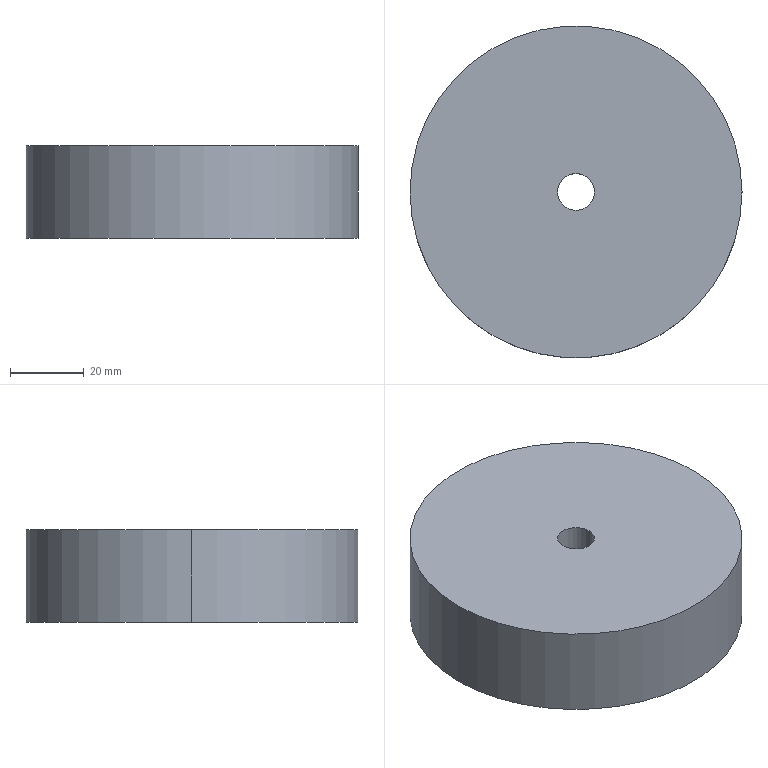Part | STEP file | 1 solid | 6 faces | box 90 x 90 x 25 mm | volume 157080 mm3 | cylinder 4 | plane 2 | commonest cylinder face diameters 10 x2 90 x2
STEP:
#1=CARTESIAN_POINT('',(0.,0.,0.));
#2=DIRECTION('',(0.,0.,1.));
#3=DIRECTION('',(1.,0.,0.));
#4=AXIS2_PLACEMENT_3D('',#1,#2,#3);
#5=CARTESIAN_POINT('',(45.,0.,0.));
#6=VERTEX_POINT('',#5);
#7=CARTESIAN_POINT('',(-45.,0.,0.));
#8=VERTEX_POINT('',#7);
#9=CARTESIAN_POINT('',(0.,0.,0.));
#10=DIRECTION('',(0.,0.,1.));
#11=DIRECTION('',(1.,0.,0.));
#12=AXIS2_PLACEMENT_3D('',#9,#10,#11);
#13=CIRCLE('',#12,45.);
#14=CARTESIAN_POINT('',(0.,0.,0.));
#15=DIRECTION('',(0.,0.,1.));
#16=DIRECTION('',(1.,0.,0.));
#17=AXIS2_PLACEMENT_3D('',#14,#15,#16);
#18=CYLINDRICAL_SURFACE('',#17,45.);
#19=CARTESIAN_POINT('',(0.,0.));
#20=DIRECTION('',(1.,0.));
#21=VECTOR('',#20,1.);
#22=LINE('',#19,#21);
#23=(GEOMETRIC_REPRESENTATION_CONTEXT(2)PARAMETRIC_REPRESENTATION_CONTEXT()REPRESENTATION_CONTEXT('',''));
#24=DEFINITIONAL_REPRESENTATION('',(#22),#23);
#25=PCURVE('',#18,#24);
#26=CARTESIAN_POINT('',(0.,0.,0.));
#27=DIRECTION('',(0.,0.,1.));
#28=DIRECTION('',(1.,0.,0.));
#29=AXIS2_PLACEMENT_3D('',#26,#27,#28);
#30=PLANE('',#29);
#31=CARTESIAN_POINT('',(0.,0.));
#32=DIRECTION('',(1.,0.));
#33=AXIS2_PLACEMENT_2D('',#31,#32);
#34=CIRCLE('',#33,45.);
#35=(GEOMETRIC_REPRESENTATION_CONTEXT(2)PARAMETRIC_REPRESENTATION_CONTEXT()REPRESENTATION_CONTEXT('',''));
#36=DEFINITIONAL_REPRESENTATION('',(#34),#35);
#37=PCURVE('',#30,#36);
#38=SURFACE_CURVE('',#13,(#25,#37),.PCURVE_S1.);
#39=EDGE_CURVE('',#6,#8,#38,.T.);
#40=ORIENTED_EDGE('',*,*,#39,.T.);
#41=CARTESIAN_POINT('',(-45.,0.,25.));
#42=VERTEX_POINT('',#41);
#43=CARTESIAN_POINT('',(-45.,0.,0.));
#44=DIRECTION('',(0.,0.,1.));
#45=VECTOR('',#44,1.);
#46=LINE('',#43,#45);
#47=CARTESIAN_POINT('',(3.142,0.));
#48=DIRECTION('',(0.,1.));
#49=VECTOR('',#48,1.);
#50=LINE('',#47,#49);
#51=(GEOMETRIC_REPRESENTATION_CONTEXT(2)PARAMETRIC_REPRESENTATION_CONTEXT()REPRESENTATION_CONTEXT('',''));
#52=DEFINITIONAL_REPRESENTATION('',(#50),#51);
#53=PCURVE('',#18,#52);
#54=CARTESIAN_POINT('',(0.,0.,0.));
#55=DIRECTION('',(0.,0.,1.));
#56=DIRECTION('',(1.,0.,0.));
#57=AXIS2_PLACEMENT_3D('',#54,#55,#56);
#58=CYLINDRICAL_SURFACE('',#57,45.);
#59=CARTESIAN_POINT('',(3.142,0.));
#60=DIRECTION('',(0.,1.));
#61=VECTOR('',#60,1.);
#62=LINE('',#59,#61);
#63=(GEOMETRIC_REPRESENTATION_CONTEXT(2)PARAMETRIC_REPRESENTATION_CONTEXT()REPRESENTATION_CONTEXT('',''));
#64=DEFINITIONAL_REPRESENTATION('',(#62),#63);
#65=PCURVE('',#58,#64);
#66=SURFACE_CURVE('',#46,(#53,#65),.PCURVE_S1.);
#67=EDGE_CURVE('',#8,#42,#66,.T.);
#68=ORIENTED_EDGE('',*,*,#67,.T.);
#69=CARTESIAN_POINT('',(45.,0.,25.));
#70=VERTEX_POINT('',#69);
#71=CARTESIAN_POINT('',(0.,0.,25.));
#72=DIRECTION('',(0.,0.,-1.));
#73=DIRECTION('',(1.,0.,0.));
#74=AXIS2_PLACEMENT_3D('',#71,#72,#73);
#75=CIRCLE('',#74,45.);
#76=CARTESIAN_POINT('',(6.283,25.));
#77=DIRECTION('',(-1.,0.));
#78=VECTOR('',#77,1.);
#79=LINE('',#76,#78);
#80=(GEOMETRIC_REPRESENTATION_CONTEXT(2)PARAMETRIC_REPRESENTATION_CONTEXT()REPRESENTATION_CONTEXT('',''));
#81=DEFINITIONAL_REPRESENTATION('',(#79),#80);
#82=PCURVE('',#18,#81);
#83=CARTESIAN_POINT('',(0.,0.,25.));
#84=DIRECTION('',(0.,0.,1.));
#85=DIRECTION('',(1.,0.,0.));
#86=AXIS2_PLACEMENT_3D('',#83,#84,#85);
#87=PLANE('',#86);
#88=CARTESIAN_POINT('',(45.,0.));
#89=CARTESIAN_POINT('',(45.,-77.942));
#90=CARTESIAN_POINT('',(-22.5,-38.971));
#91=CARTESIAN_POINT('',(-90.,0.));
#92=CARTESIAN_POINT('',(-22.5,38.971));
#93=CARTESIAN_POINT('',(45.,77.942));
#94=CARTESIAN_POINT('',(45.,0.));
#95=(BOUNDED_CURVE()B_SPLINE_CURVE(2,(#88,#89,#90,#91,#92,#93,#94),.UNSPECIFIED.,.T.,.F.)B_SPLINE_CURVE_WITH_KNOTS((1,2,2,2,2,1),(-2.094,0.,2.094,4.189,6.283,8.378),.UNSPECIFIED.)CURVE()GEOMETRIC_REPRESENTATION_ITEM()RATIONAL_B_SPLINE_CURVE((1.,0.5,1.,0.5,1.,0.5,1.))REPRESENTATION_ITEM(''));
#96=(GEOMETRIC_REPRESENTATION_CONTEXT(2)PARAMETRIC_REPRESENTATION_CONTEXT()REPRESENTATION_CONTEXT('',''));
#97=DEFINITIONAL_REPRESENTATION('',(#95),#96);
#98=PCURVE('',#87,#97);
#99=SURFACE_CURVE('',#75,(#82,#98),.PCURVE_S1.);
#100=EDGE_CURVE('',#42,#70,#99,.T.);
#101=ORIENTED_EDGE('',*,*,#100,.T.);
#102=CARTESIAN_POINT('',(45.,0.,0.));
#103=DIRECTION('',(0.,0.,1.));
#104=VECTOR('',#103,1.);
#105=LINE('',#102,#104);
#106=CARTESIAN_POINT('',(0.,0.));
#107=DIRECTION('',(0.,1.));
#108=VECTOR('',#107,1.);
#109=LINE('',#106,#108);
#110=(GEOMETRIC_REPRESENTATION_CONTEXT(2)PARAMETRIC_REPRESENTATION_CONTEXT()REPRESENTATION_CONTEXT('',''));
#111=DEFINITIONAL_REPRESENTATION('',(#109),#110);
#112=PCURVE('',#18,#111);
#113=CARTESIAN_POINT('',(6.283,0.));
#114=DIRECTION('',(0.,1.));
#115=VECTOR('',#114,1.);
#116=LINE('',#113,#115);
#117=(GEOMETRIC_REPRESENTATION_CONTEXT(2)PARAMETRIC_REPRESENTATION_CONTEXT()REPRESENTATION_CONTEXT('',''));
#118=DEFINITIONAL_REPRESENTATION('',(#116),#117);
#119=PCURVE('',#58,#118);
#120=SURFACE_CURVE('',#105,(#112,#119),.PCURVE_S1.);
#121=EDGE_CURVE('',#6,#70,#120,.T.);
#122=ORIENTED_EDGE('',*,*,#121,.F.);
#123=EDGE_LOOP('',(#40,#68,#101,#122));
#124=FACE_BOUND('',#123,.T.);
#125=ADVANCED_FACE('',(#124),#18,.T.);
#126=CARTESIAN_POINT('',(-5.,0.,25.));
#127=VERTEX_POINT('',#126);
#128=CARTESIAN_POINT('',(-5.,0.,0.));
#129=VERTEX_POINT('',#128);
#130=CARTESIAN_POINT('',(-5.,0.,25.));
#131=DIRECTION('',(0.,0.,-1.));
#132=VECTOR('',#131,1.);
#133=LINE('',#130,#132);
#134=CARTESIAN_POINT('',(0.,0.,25.));
#135=DIRECTION('',(0.,0.,-1.));
#136=DIRECTION('',(-1.,0.,0.));
#137=AXIS2_PLACEMENT_3D('',#134,#135,#136);
#138=CYLINDRICAL_SURFACE('',#137,5.);
#139=CARTESIAN_POINT('',(6.283,0.));
#140=DIRECTION('',(0.,1.));
#141=VECTOR('',#140,1.);
#142=LINE('',#139,#141);
#143=(GEOMETRIC_REPRESENTATION_CONTEXT(2)PARAMETRIC_REPRESENTATION_CONTEXT()REPRESENTATION_CONTEXT('',''));
#144=DEFINITIONAL_REPRESENTATION('',(#142),#143);
#145=PCURVE('',#138,#144);
#146=CARTESIAN_POINT('',(0.,0.,25.));
#147=DIRECTION('',(0.,0.,-1.));
#148=DIRECTION('',(-1.,0.,0.));
#149=AXIS2_PLACEMENT_3D('',#146,#147,#148);
#150=CYLINDRICAL_SURFACE('',#149,5.);
#151=CARTESIAN_POINT('',(0.,0.));
#152=DIRECTION('',(0.,1.));
#153=VECTOR('',#152,1.);
#154=LINE('',#151,#153);
#155=(GEOMETRIC_REPRESENTATION_CONTEXT(2)PARAMETRIC_REPRESENTATION_CONTEXT()REPRESENTATION_CONTEXT('',''));
#156=DEFINITIONAL_REPRESENTATION('',(#154),#155);
#157=PCURVE('',#150,#156);
#158=SURFACE_CURVE('',#133,(#145,#157),.PCURVE_S1.);
#159=EDGE_CURVE('',#127,#129,#158,.T.);
#160=ORIENTED_EDGE('',*,*,#159,.T.);
#161=CARTESIAN_POINT('',(5.,0.,0.));
#162=VERTEX_POINT('',#161);
#163=CARTESIAN_POINT('',(0.,0.,0.));
#164=DIRECTION('',(0.,0.,-1.));
#165=DIRECTION('',(-1.,0.,0.));
#166=AXIS2_PLACEMENT_3D('',#163,#164,#165);
#167=CIRCLE('',#166,5.);
#168=CARTESIAN_POINT('',(0.,25.));
#169=DIRECTION('',(1.,0.));
#170=VECTOR('',#169,1.);
#171=LINE('',#168,#170);
#172=(GEOMETRIC_REPRESENTATION_CONTEXT(2)PARAMETRIC_REPRESENTATION_CONTEXT()REPRESENTATION_CONTEXT('',''));
#173=DEFINITIONAL_REPRESENTATION('',(#171),#172);
#174=PCURVE('',#138,#173);
#175=CARTESIAN_POINT('',(-5.,0.));
#176=CARTESIAN_POINT('',(-5.,8.66));
#177=CARTESIAN_POINT('',(2.5,4.33));
#178=CARTESIAN_POINT('',(10.,0.));
#179=CARTESIAN_POINT('',(2.5,-4.33));
#180=CARTESIAN_POINT('',(-5.,-8.66));
#181=CARTESIAN_POINT('',(-5.,0.));
#182=(BOUNDED_CURVE()B_SPLINE_CURVE(2,(#175,#176,#177,#178,#179,#180,#181),.UNSPECIFIED.,.T.,.F.)B_SPLINE_CURVE_WITH_KNOTS((1,2,2,2,2,1),(-2.094,0.,2.094,4.189,6.283,8.378),.UNSPECIFIED.)CURVE()GEOMETRIC_REPRESENTATION_ITEM()RATIONAL_B_SPLINE_CURVE((1.,0.5,1.,0.5,1.,0.5,1.))REPRESENTATION_ITEM(''));
#183=(GEOMETRIC_REPRESENTATION_CONTEXT(2)PARAMETRIC_REPRESENTATION_CONTEXT()REPRESENTATION_CONTEXT('',''));
#184=DEFINITIONAL_REPRESENTATION('',(#182),#183);
#185=PCURVE('',#30,#184);
#186=SURFACE_CURVE('',#167,(#174,#185),.PCURVE_S1.);
#187=EDGE_CURVE('',#162,#129,#186,.T.);
#188=ORIENTED_EDGE('',*,*,#187,.F.);
#189=CARTESIAN_POINT('',(5.,0.,25.));
#190=VERTEX_POINT('',#189);
#191=CARTESIAN_POINT('',(5.,0.,25.));
#192=DIRECTION('',(0.,0.,-1.));
#193=VECTOR('',#192,1.);
#194=LINE('',#191,#193);
#195=CARTESIAN_POINT('',(3.142,0.));
#196=DIRECTION('',(0.,1.));
#197=VECTOR('',#196,1.);
#198=LINE('',#195,#197);
#199=(GEOMETRIC_REPRESENTATION_CONTEXT(2)PARAMETRIC_REPRESENTATION_CONTEXT()REPRESENTATION_CONTEXT('',''));
#200=DEFINITIONAL_REPRESENTATION('',(#198),#199);
#201=PCURVE('',#138,#200);
#202=CARTESIAN_POINT('',(3.142,0.));
#203=DIRECTION('',(0.,1.));
#204=VECTOR('',#203,1.);
#205=LINE('',#202,#204);
#206=(GEOMETRIC_REPRESENTATION_CONTEXT(2)PARAMETRIC_REPRESENTATION_CONTEXT()REPRESENTATION_CONTEXT('',''));
#207=DEFINITIONAL_REPRESENTATION('',(#205),#206);
#208=PCURVE('',#150,#207);
#209=SURFACE_CURVE('',#194,(#201,#208),.PCURVE_S1.);
#210=EDGE_CURVE('',#190,#162,#209,.T.);
#211=ORIENTED_EDGE('',*,*,#210,.F.);
#212=CARTESIAN_POINT('',(0.,0.,25.));
#213=DIRECTION('',(0.,0.,-1.));
#214=DIRECTION('',(-1.,0.,0.));
#215=AXIS2_PLACEMENT_3D('',#212,#213,#214);
#216=CIRCLE('',#215,5.);
#217=CARTESIAN_POINT('',(0.,0.));
#218=DIRECTION('',(1.,0.));
#219=VECTOR('',#218,1.);
#220=LINE('',#217,#219);
#221=(GEOMETRIC_REPRESENTATION_CONTEXT(2)PARAMETRIC_REPRESENTATION_CONTEXT()REPRESENTATION_CONTEXT('',''));
#222=DEFINITIONAL_REPRESENTATION('',(#220),#221);
#223=PCURVE('',#138,#222);
#224=CARTESIAN_POINT('',(-5.,0.));
#225=CARTESIAN_POINT('',(-5.,8.66));
#226=CARTESIAN_POINT('',(2.5,4.33));
#227=CARTESIAN_POINT('',(10.,0.));
#228=CARTESIAN_POINT('',(2.5,-4.33));
#229=CARTESIAN_POINT('',(-5.,-8.66));
#230=CARTESIAN_POINT('',(-5.,0.));
#231=(BOUNDED_CURVE()B_SPLINE_CURVE(2,(#224,#225,#226,#227,#228,#229,#230),.UNSPECIFIED.,.T.,.F.)B_SPLINE_CURVE_WITH_KNOTS((1,2,2,2,2,1),(-2.094,0.,2.094,4.189,6.283,8.378),.UNSPECIFIED.)CURVE()GEOMETRIC_REPRESENTATION_ITEM()RATIONAL_B_SPLINE_CURVE((1.,0.5,1.,0.5,1.,0.5,1.))REPRESENTATION_ITEM(''));
#232=(GEOMETRIC_REPRESENTATION_CONTEXT(2)PARAMETRIC_REPRESENTATION_CONTEXT()REPRESENTATION_CONTEXT('',''));
#233=DEFINITIONAL_REPRESENTATION('',(#231),#232);
#234=PCURVE('',#87,#233);
#235=SURFACE_CURVE('',#216,(#223,#234),.PCURVE_S1.);
#236=EDGE_CURVE('',#190,#127,#235,.T.);
#237=ORIENTED_EDGE('',*,*,#236,.T.);
#238=EDGE_LOOP('',(#160,#188,#211,#237));
#239=FACE_BOUND('',#238,.F.);
#240=ADVANCED_FACE('',(#239),#138,.F.);
#241=ORIENTED_EDGE('',*,*,#67,.F.);
#242=CARTESIAN_POINT('',(0.,0.,0.));
#243=DIRECTION('',(0.,0.,1.));
#244=DIRECTION('',(1.,0.,0.));
#245=AXIS2_PLACEMENT_3D('',#242,#243,#244);
#246=CIRCLE('',#245,45.);
#247=CARTESIAN_POINT('',(0.,0.));
#248=DIRECTION('',(1.,0.));
#249=VECTOR('',#248,1.);
#250=LINE('',#247,#249);
#251=(GEOMETRIC_REPRESENTATION_CONTEXT(2)PARAMETRIC_REPRESENTATION_CONTEXT()REPRESENTATION_CONTEXT('',''));
#252=DEFINITIONAL_REPRESENTATION('',(#250),#251);
#253=PCURVE('',#58,#252);
#254=CARTESIAN_POINT('',(0.,0.));
#255=DIRECTION('',(1.,0.));
#256=AXIS2_PLACEMENT_2D('',#254,#255);
#257=CIRCLE('',#256,45.);
#258=(GEOMETRIC_REPRESENTATION_CONTEXT(2)PARAMETRIC_REPRESENTATION_CONTEXT()REPRESENTATION_CONTEXT('',''));
#259=DEFINITIONAL_REPRESENTATION('',(#257),#258);
#260=PCURVE('',#30,#259);
#261=SURFACE_CURVE('',#246,(#253,#260),.PCURVE_S1.);
#262=EDGE_CURVE('',#8,#6,#261,.T.);
#263=ORIENTED_EDGE('',*,*,#262,.T.);
#264=ORIENTED_EDGE('',*,*,#121,.T.);
#265=CARTESIAN_POINT('',(0.,0.,25.));
#266=DIRECTION('',(0.,0.,-1.));
#267=DIRECTION('',(1.,0.,0.));
#268=AXIS2_PLACEMENT_3D('',#265,#266,#267);
#269=CIRCLE('',#268,45.);
#270=CARTESIAN_POINT('',(6.283,25.));
#271=DIRECTION('',(-1.,0.));
#272=VECTOR('',#271,1.);
#273=LINE('',#270,#272);
#274=(GEOMETRIC_REPRESENTATION_CONTEXT(2)PARAMETRIC_REPRESENTATION_CONTEXT()REPRESENTATION_CONTEXT('',''));
#275=DEFINITIONAL_REPRESENTATION('',(#273),#274);
#276=PCURVE('',#58,#275);
#277=CARTESIAN_POINT('',(45.,0.));
#278=CARTESIAN_POINT('',(45.,-77.942));
#279=CARTESIAN_POINT('',(-22.5,-38.971));
#280=CARTESIAN_POINT('',(-90.,0.));
#281=CARTESIAN_POINT('',(-22.5,38.971));
#282=CARTESIAN_POINT('',(45.,77.942));
#283=CARTESIAN_POINT('',(45.,0.));
#284=(BOUNDED_CURVE()B_SPLINE_CURVE(2,(#277,#278,#279,#280,#281,#282,#283),.UNSPECIFIED.,.T.,.F.)B_SPLINE_CURVE_WITH_KNOTS((1,2,2,2,2,1),(-2.094,0.,2.094,4.189,6.283,8.378),.UNSPECIFIED.)CURVE()GEOMETRIC_REPRESENTATION_ITEM()RATIONAL_B_SPLINE_CURVE((1.,0.5,1.,0.5,1.,0.5,1.))REPRESENTATION_ITEM(''));
#285=(GEOMETRIC_REPRESENTATION_CONTEXT(2)PARAMETRIC_REPRESENTATION_CONTEXT()REPRESENTATION_CONTEXT('',''));
#286=DEFINITIONAL_REPRESENTATION('',(#284),#285);
#287=PCURVE('',#87,#286);
#288=SURFACE_CURVE('',#269,(#276,#287),.PCURVE_S1.);
#289=EDGE_CURVE('',#70,#42,#288,.T.);
#290=ORIENTED_EDGE('',*,*,#289,.T.);
#291=EDGE_LOOP('',(#241,#263,#264,#290));
#292=FACE_BOUND('',#291,.T.);
#293=ADVANCED_FACE('',(#292),#58,.T.);
#294=ORIENTED_EDGE('',*,*,#39,.F.);
#295=ORIENTED_EDGE('',*,*,#262,.F.);
#296=EDGE_LOOP('',(#294,#295));
#297=FACE_BOUND('',#296,.T.);
#298=CARTESIAN_POINT('',(0.,0.,0.));
#299=DIRECTION('',(0.,0.,-1.));
#300=DIRECTION('',(-1.,0.,0.));
#301=AXIS2_PLACEMENT_3D('',#298,#299,#300);
#302=CIRCLE('',#301,5.);
#303=CARTESIAN_POINT('',(-5.,0.));
#304=CARTESIAN_POINT('',(-5.,8.66));
#305=CARTESIAN_POINT('',(2.5,4.33));
#306=CARTESIAN_POINT('',(10.,0.));
#307=CARTESIAN_POINT('',(2.5,-4.33));
#308=CARTESIAN_POINT('',(-5.,-8.66));
#309=CARTESIAN_POINT('',(-5.,0.));
#310=(BOUNDED_CURVE()B_SPLINE_CURVE(2,(#303,#304,#305,#306,#307,#308,#309),.UNSPECIFIED.,.T.,.F.)B_SPLINE_CURVE_WITH_KNOTS((1,2,2,2,2,1),(-2.094,0.,2.094,4.189,6.283,8.378),.UNSPECIFIED.)CURVE()GEOMETRIC_REPRESENTATION_ITEM()RATIONAL_B_SPLINE_CURVE((1.,0.5,1.,0.5,1.,0.5,1.))REPRESENTATION_ITEM(''));
#311=(GEOMETRIC_REPRESENTATION_CONTEXT(2)PARAMETRIC_REPRESENTATION_CONTEXT()REPRESENTATION_CONTEXT('',''));
#312=DEFINITIONAL_REPRESENTATION('',(#310),#311);
#313=PCURVE('',#30,#312);
#314=CARTESIAN_POINT('',(0.,25.));
#315=DIRECTION('',(1.,0.));
#316=VECTOR('',#315,1.);
#317=LINE('',#314,#316);
#318=(GEOMETRIC_REPRESENTATION_CONTEXT(2)PARAMETRIC_REPRESENTATION_CONTEXT()REPRESENTATION_CONTEXT('',''));
#319=DEFINITIONAL_REPRESENTATION('',(#317),#318);
#320=PCURVE('',#150,#319);
#321=SURFACE_CURVE('',#302,(#313,#320),.PCURVE_S1.);
#322=EDGE_CURVE('',#129,#162,#321,.T.);
#323=ORIENTED_EDGE('',*,*,#322,.F.);
#324=ORIENTED_EDGE('',*,*,#187,.F.);
#325=EDGE_LOOP('',(#323,#324));
#326=FACE_BOUND('',#325,.T.);
#327=ADVANCED_FACE('',(#297,#326),#30,.F.);
#328=ORIENTED_EDGE('',*,*,#289,.F.);
#329=ORIENTED_EDGE('',*,*,#100,.F.);
#330=EDGE_LOOP('',(#328,#329));
#331=FACE_BOUND('',#330,.T.);
#332=CARTESIAN_POINT('',(0.,0.,25.));
#333=DIRECTION('',(0.,0.,-1.));
#334=DIRECTION('',(-1.,0.,0.));
#335=AXIS2_PLACEMENT_3D('',#332,#333,#334);
#336=CIRCLE('',#335,5.);
#337=CARTESIAN_POINT('',(-5.,0.));
#338=CARTESIAN_POINT('',(-5.,8.66));
#339=CARTESIAN_POINT('',(2.5,4.33));
#340=CARTESIAN_POINT('',(10.,0.));
#341=CARTESIAN_POINT('',(2.5,-4.33));
#342=CARTESIAN_POINT('',(-5.,-8.66));
#343=CARTESIAN_POINT('',(-5.,0.));
#344=(BOUNDED_CURVE()B_SPLINE_CURVE(2,(#337,#338,#339,#340,#341,#342,#343),.UNSPECIFIED.,.T.,.F.)B_SPLINE_CURVE_WITH_KNOTS((1,2,2,2,2,1),(-2.094,0.,2.094,4.189,6.283,8.378),.UNSPECIFIED.)CURVE()GEOMETRIC_REPRESENTATION_ITEM()RATIONAL_B_SPLINE_CURVE((1.,0.5,1.,0.5,1.,0.5,1.))REPRESENTATION_ITEM(''));
#345=(GEOMETRIC_REPRESENTATION_CONTEXT(2)PARAMETRIC_REPRESENTATION_CONTEXT()REPRESENTATION_CONTEXT('',''));
#346=DEFINITIONAL_REPRESENTATION('',(#344),#345);
#347=PCURVE('',#87,#346);
#348=CARTESIAN_POINT('',(0.,0.));
#349=DIRECTION('',(1.,0.));
#350=VECTOR('',#349,1.);
#351=LINE('',#348,#350);
#352=(GEOMETRIC_REPRESENTATION_CONTEXT(2)PARAMETRIC_REPRESENTATION_CONTEXT()REPRESENTATION_CONTEXT('',''));
#353=DEFINITIONAL_REPRESENTATION('',(#351),#352);
#354=PCURVE('',#150,#353);
#355=SURFACE_CURVE('',#336,(#347,#354),.PCURVE_S1.);
#356=EDGE_CURVE('',#127,#190,#355,.T.);
#357=ORIENTED_EDGE('',*,*,#356,.T.);
#358=ORIENTED_EDGE('',*,*,#236,.T.);
#359=EDGE_LOOP('',(#357,#358));
#360=FACE_BOUND('',#359,.T.);
#361=ADVANCED_FACE('',(#331,#360),#87,.T.);
#362=ORIENTED_EDGE('',*,*,#322,.F.);
#363=ORIENTED_EDGE('',*,*,#159,.F.);
#364=ORIENTED_EDGE('',*,*,#356,.T.);
#365=ORIENTED_EDGE('',*,*,#210,.T.);
#366=EDGE_LOOP('',(#362,#363,#364,#365));
#367=FACE_BOUND('',#366,.F.);
#368=ADVANCED_FACE('',(#367),#150,.F.);
#369=CLOSED_SHELL('',(#125,#240,#293,#327,#361,#368));
#370=MANIFOLD_SOLID_BREP('',#369);
#371=(LENGTH_UNIT()NAMED_UNIT(*)SI_UNIT(.MILLI.,.METRE.));
#372=UNCERTAINTY_MEASURE_WITH_UNIT(LENGTH_MEASURE(0.0000001),#371,'','');
#373=(NAMED_UNIT(*)PLANE_ANGLE_UNIT()SI_UNIT($,.RADIAN.));
#374=(NAMED_UNIT(*)SI_UNIT($,.STERADIAN.)SOLID_ANGLE_UNIT());
#375=(GEOMETRIC_REPRESENTATION_CONTEXT(3)GLOBAL_UNCERTAINTY_ASSIGNED_CONTEXT((#372))GLOBAL_UNIT_ASSIGNED_CONTEXT((#371,#373,#374))REPRESENTATION_CONTEXT('',''));
#376=ADVANCED_BREP_SHAPE_REPRESENTATION('',(#4,#370),#375);